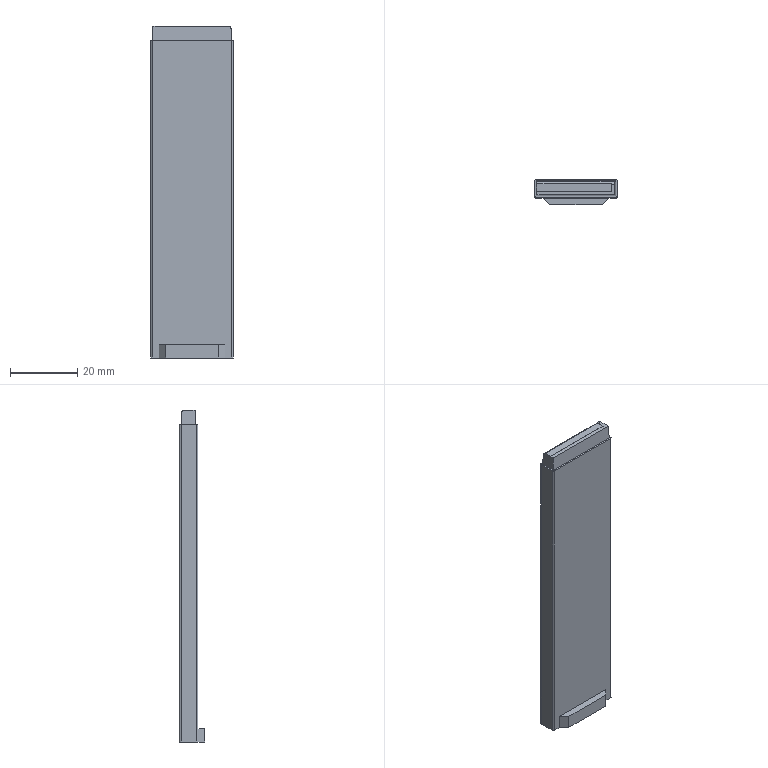Part | Creo | 1 solid | 23 faces | box 24.5 x 7.5 x 98.442 mm | volume 13224 mm3 | plane 18 | cylinder 5 | commonest cylinder face diameters 1 x4 2.01 x1
STEP:
#1=CARTESIAN_POINT('',(0.,0.,0.));
#2=DIRECTION('',(0.,0.,1.));
#3=DIRECTION('',(1.,0.,0.));
#4=AXIS2_PLACEMENT_3D('',#1,#2,#3);
#5=CARTESIAN_POINT('',(-20.598,-39.362,-54.09));
#6=VERTEX_POINT('',#5);
#7=CARTESIAN_POINT('',(-36.098,-39.362,-54.09));
#8=VERTEX_POINT('',#7);
#9=CARTESIAN_POINT('',(-20.598,-39.362,-54.09));
#10=DIRECTION('',(-1.,0.,0.));
#11=VECTOR('',#10,15.5);
#12=LINE('',#9,#11);
#13=EDGE_CURVE('',#6,#8,#12,.T.);
#14=ORIENTED_EDGE('',*,*,#13,.F.);
#15=CARTESIAN_POINT('',(-18.598,-37.362,-54.09));
#16=VERTEX_POINT('',#15);
#17=CARTESIAN_POINT('',(-18.598,-37.362,-54.09));
#18=DIRECTION('',(-0.7071,-0.7071,0.));
#19=VECTOR('',#18,2.828);
#20=LINE('',#17,#19);
#21=EDGE_CURVE('',#16,#6,#20,.T.);
#22=ORIENTED_EDGE('',*,*,#21,.F.);
#23=CARTESIAN_POINT('',(-16.598,-37.362,-54.09));
#24=VERTEX_POINT('',#23);
#25=CARTESIAN_POINT('',(-16.598,-37.362,-54.09));
#26=DIRECTION('',(-1.,0.,0.));
#27=VECTOR('',#26,2.);
#28=LINE('',#25,#27);
#29=EDGE_CURVE('',#24,#16,#28,.T.);
#30=ORIENTED_EDGE('',*,*,#29,.F.);
#31=CARTESIAN_POINT('',(-16.098,-36.862,-54.09));
#32=VERTEX_POINT('',#31);
#33=CARTESIAN_POINT('',(-16.598,-36.862,-54.09));
#34=DIRECTION('',(0.,0.,-1.));
#35=DIRECTION('',(1.,0.,0.));
#36=AXIS2_PLACEMENT_3D('',#33,#34,#35);
#37=CIRCLE('',#36,0.5);
#38=EDGE_CURVE('',#32,#24,#37,.T.);
#39=ORIENTED_EDGE('',*,*,#38,.F.);
#40=CARTESIAN_POINT('',(-16.098,-32.362,-54.09));
#41=VERTEX_POINT('',#40);
#42=CARTESIAN_POINT('',(-16.098,-32.362,-54.09));
#43=DIRECTION('',(0.,-1.,0.));
#44=VECTOR('',#43,4.5);
#45=LINE('',#42,#44);
#46=EDGE_CURVE('',#41,#32,#45,.T.);
#47=ORIENTED_EDGE('',*,*,#46,.F.);
#48=CARTESIAN_POINT('',(-16.598,-31.862,-54.09));
#49=VERTEX_POINT('',#48);
#50=CARTESIAN_POINT('',(-16.598,-32.362,-54.09));
#51=DIRECTION('',(0.,0.,-1.));
#52=DIRECTION('',(0.,1.,0.));
#53=AXIS2_PLACEMENT_3D('',#50,#51,#52);
#54=CIRCLE('',#53,0.5);
#55=EDGE_CURVE('',#49,#41,#54,.T.);
#56=ORIENTED_EDGE('',*,*,#55,.F.);
#57=CARTESIAN_POINT('',(-40.098,-31.862,-54.09));
#58=VERTEX_POINT('',#57);
#59=CARTESIAN_POINT('',(-40.098,-31.862,-54.09));
#60=DIRECTION('',(1.,0.,0.));
#61=VECTOR('',#60,23.5);
#62=LINE('',#59,#61);
#63=EDGE_CURVE('',#58,#49,#62,.T.);
#64=ORIENTED_EDGE('',*,*,#63,.F.);
#65=CARTESIAN_POINT('',(-40.598,-32.362,-54.09));
#66=VERTEX_POINT('',#65);
#67=CARTESIAN_POINT('',(-40.098,-32.362,-54.09));
#68=DIRECTION('',(0.,0.,-1.));
#69=DIRECTION('',(-1.,0.,0.));
#70=AXIS2_PLACEMENT_3D('',#67,#68,#69);
#71=CIRCLE('',#70,0.5);
#72=EDGE_CURVE('',#66,#58,#71,.T.);
#73=ORIENTED_EDGE('',*,*,#72,.F.);
#74=CARTESIAN_POINT('',(-40.598,-36.862,-54.09));
#75=VERTEX_POINT('',#74);
#76=CARTESIAN_POINT('',(-40.598,-36.862,-54.09));
#77=DIRECTION('',(0.,1.,0.));
#78=VECTOR('',#77,4.5);
#79=LINE('',#76,#78);
#80=EDGE_CURVE('',#75,#66,#79,.T.);
#81=ORIENTED_EDGE('',*,*,#80,.F.);
#82=CARTESIAN_POINT('',(-40.098,-37.362,-54.09));
#83=VERTEX_POINT('',#82);
#84=CARTESIAN_POINT('',(-40.098,-36.862,-54.09));
#85=DIRECTION('',(0.,0.,-1.));
#86=DIRECTION('',(0.,-1.,0.));
#87=AXIS2_PLACEMENT_3D('',#84,#85,#86);
#88=CIRCLE('',#87,0.5);
#89=EDGE_CURVE('',#83,#75,#88,.T.);
#90=ORIENTED_EDGE('',*,*,#89,.F.);
#91=CARTESIAN_POINT('',(-38.098,-37.362,-54.09));
#92=VERTEX_POINT('',#91);
#93=CARTESIAN_POINT('',(-38.098,-37.362,-54.09));
#94=DIRECTION('',(-1.,0.,0.));
#95=VECTOR('',#94,2.);
#96=LINE('',#93,#95);
#97=EDGE_CURVE('',#92,#83,#96,.T.);
#98=ORIENTED_EDGE('',*,*,#97,.F.);
#99=CARTESIAN_POINT('',(-36.098,-39.362,-54.09));
#100=DIRECTION('',(-0.7071,0.7071,0.));
#101=VECTOR('',#100,2.828);
#102=LINE('',#99,#101);
#103=EDGE_CURVE('',#8,#92,#102,.T.);
#104=ORIENTED_EDGE('',*,*,#103,.F.);
#105=EDGE_LOOP('',(#14,#22,#30,#39,#47,#56,#64,#73,#81,#90,#98,#104));
#106=FACE_OUTER_BOUND('',#105,.F.);
#107=CARTESIAN_POINT('',(0.,0.,-54.09));
#108=DIRECTION('',(0.,0.,-1.));
#109=DIRECTION('',(-1.,0.,0.));
#110=AXIS2_PLACEMENT_3D('',#107,#108,#109);
#111=PLANE('',#110);
#112=ADVANCED_FACE('',(#106),#111,.T.);
#113=CARTESIAN_POINT('',(-36.098,-39.362,-50.09));
#114=VERTEX_POINT('',#113);
#115=CARTESIAN_POINT('',(-20.598,-39.362,-50.09));
#116=VERTEX_POINT('',#115);
#117=CARTESIAN_POINT('',(-36.098,-39.362,-50.09));
#118=DIRECTION('',(1.,0.,0.));
#119=VECTOR('',#118,15.5);
#120=LINE('',#117,#119);
#121=EDGE_CURVE('',#114,#116,#120,.T.);
#122=ORIENTED_EDGE('',*,*,#121,.T.);
#123=CARTESIAN_POINT('',(-20.598,-39.362,-50.09));
#124=DIRECTION('',(0.,0.,-1.));
#125=VECTOR('',#124,4.);
#126=LINE('',#123,#125);
#127=EDGE_CURVE('',#116,#6,#126,.T.);
#128=ORIENTED_EDGE('',*,*,#127,.T.);
#129=ORIENTED_EDGE('',*,*,#13,.T.);
#130=CARTESIAN_POINT('',(-36.098,-39.362,-54.09));
#131=DIRECTION('',(0.,0.,1.));
#132=VECTOR('',#131,4.);
#133=LINE('',#130,#132);
#134=EDGE_CURVE('',#8,#114,#133,.T.);
#135=ORIENTED_EDGE('',*,*,#134,.T.);
#136=EDGE_LOOP('',(#122,#128,#129,#135));
#137=FACE_OUTER_BOUND('',#136,.F.);
#138=CARTESIAN_POINT('',(-28.348,-39.362,-54.09));
#139=DIRECTION('',(0.,-1.,0.));
#140=DIRECTION('',(0.,0.,-1.));
#141=AXIS2_PLACEMENT_3D('',#138,#139,#140);
#142=PLANE('',#141);
#143=ADVANCED_FACE('',(#137),#142,.T.);
#144=CARTESIAN_POINT('',(-18.598,-37.362,-50.09));
#145=VERTEX_POINT('',#144);
#146=CARTESIAN_POINT('',(-38.098,-37.362,-50.09));
#147=VERTEX_POINT('',#146);
#148=CARTESIAN_POINT('',(-18.598,-37.362,-50.09));
#149=DIRECTION('',(-1.,0.,0.));
#150=VECTOR('',#149,19.5);
#151=LINE('',#148,#150);
#152=EDGE_CURVE('',#145,#147,#151,.T.);
#153=ORIENTED_EDGE('',*,*,#152,.F.);
#154=CARTESIAN_POINT('',(-20.598,-39.362,-50.09));
#155=DIRECTION('',(0.7071,0.7071,0.));
#156=VECTOR('',#155,2.828);
#157=LINE('',#154,#156);
#158=EDGE_CURVE('',#116,#145,#157,.T.);
#159=ORIENTED_EDGE('',*,*,#158,.F.);
#160=ORIENTED_EDGE('',*,*,#121,.F.);
#161=CARTESIAN_POINT('',(-38.098,-37.362,-50.09));
#162=DIRECTION('',(0.7071,-0.7071,0.));
#163=VECTOR('',#162,2.828);
#164=LINE('',#161,#163);
#165=EDGE_CURVE('',#147,#114,#164,.T.);
#166=ORIENTED_EDGE('',*,*,#165,.F.);
#167=EDGE_LOOP('',(#153,#159,#160,#166));
#168=FACE_OUTER_BOUND('',#167,.F.);
#169=CARTESIAN_POINT('',(-28.348,-37.862,-50.09));
#170=DIRECTION('',(0.,0.,1.));
#171=DIRECTION('',(1.,0.,0.));
#172=AXIS2_PLACEMENT_3D('',#169,#170,#171);
#173=PLANE('',#172);
#174=ADVANCED_FACE('',(#168),#173,.T.);
#175=ORIENTED_EDGE('',*,*,#97,.T.);
#176=CARTESIAN_POINT('',(-40.098,-37.362,40.081));
#177=VERTEX_POINT('',#176);
#178=CARTESIAN_POINT('',(-40.098,-37.362,-54.09));
#179=DIRECTION('',(0.,0.,1.));
#180=VECTOR('',#179,94.171);
#181=LINE('',#178,#180);
#182=EDGE_CURVE('',#83,#177,#181,.T.);
#183=ORIENTED_EDGE('',*,*,#182,.T.);
#184=CARTESIAN_POINT('',(-16.598,-37.362,40.081));
#185=VERTEX_POINT('',#184);
#186=CARTESIAN_POINT('',(-40.098,-37.362,40.081));
#187=DIRECTION('',(1.,0.,0.));
#188=VECTOR('',#187,23.5);
#189=LINE('',#186,#188);
#190=EDGE_CURVE('',#177,#185,#189,.T.);
#191=ORIENTED_EDGE('',*,*,#190,.T.);
#192=CARTESIAN_POINT('',(-16.598,-37.362,40.081));
#193=DIRECTION('',(0.,0.,-1.));
#194=VECTOR('',#193,94.171);
#195=LINE('',#192,#194);
#196=EDGE_CURVE('',#185,#24,#195,.T.);
#197=ORIENTED_EDGE('',*,*,#196,.T.);
#198=ORIENTED_EDGE('',*,*,#29,.T.);
#199=CARTESIAN_POINT('',(-18.598,-37.362,-54.09));
#200=DIRECTION('',(0.,0.,1.));
#201=VECTOR('',#200,4.);
#202=LINE('',#199,#201);
#203=EDGE_CURVE('',#16,#145,#202,.T.);
#204=ORIENTED_EDGE('',*,*,#203,.T.);
#205=ORIENTED_EDGE('',*,*,#152,.T.);
#206=CARTESIAN_POINT('',(-38.098,-37.362,-50.09));
#207=DIRECTION('',(0.,0.,-1.));
#208=VECTOR('',#207,4.);
#209=LINE('',#206,#208);
#210=EDGE_CURVE('',#147,#92,#209,.T.);
#211=ORIENTED_EDGE('',*,*,#210,.T.);
#212=EDGE_LOOP('',(#175,#183,#191,#197,#198,#204,#205,#211));
#213=FACE_OUTER_BOUND('',#212,.F.);
#214=CARTESIAN_POINT('',(-40.598,-37.362,68.91));
#215=DIRECTION('',(0.,1.,0.));
#216=DIRECTION('',(0.,0.,1.));
#217=AXIS2_PLACEMENT_3D('',#214,#215,#216);
#218=PLANE('',#217);
#219=ADVANCED_FACE('',(#213),#218,.F.);
#220=CARTESIAN_POINT('',(-40.598,-36.862,40.081));
#221=VERTEX_POINT('',#220);
#222=CARTESIAN_POINT('',(-40.098,-36.862,40.081));
#223=DIRECTION('',(0.,0.,1.));
#224=DIRECTION('',(-1.,0.,0.));
#225=AXIS2_PLACEMENT_3D('',#222,#223,#224);
#226=CIRCLE('',#225,0.5);
#227=EDGE_CURVE('',#221,#177,#226,.T.);
#228=ORIENTED_EDGE('',*,*,#227,.T.);
#229=ORIENTED_EDGE('',*,*,#182,.F.);
#230=ORIENTED_EDGE('',*,*,#89,.T.);
#231=CARTESIAN_POINT('',(-40.598,-36.862,40.081));
#232=DIRECTION('',(0.,0.,-1.));
#233=VECTOR('',#232,94.171);
#234=LINE('',#231,#233);
#235=EDGE_CURVE('',#221,#75,#234,.T.);
#236=ORIENTED_EDGE('',*,*,#235,.F.);
#237=EDGE_LOOP('',(#228,#229,#230,#236));
#238=FACE_OUTER_BOUND('',#237,.F.);
#239=CARTESIAN_POINT('',(-40.098,-36.862,68.91));
#240=DIRECTION('',(0.,0.,-1.));
#241=DIRECTION('',(-1.,0.,0.));
#242=AXIS2_PLACEMENT_3D('',#239,#240,#241);
#243=CYLINDRICAL_SURFACE('',#242,0.5);
#244=ADVANCED_FACE('',(#238),#243,.T.);
#245=CARTESIAN_POINT('',(-16.598,-31.862,40.081));
#246=VERTEX_POINT('',#245);
#247=CARTESIAN_POINT('',(-40.098,-31.862,40.081));
#248=VERTEX_POINT('',#247);
#249=CARTESIAN_POINT('',(-16.598,-31.862,40.081));
#250=DIRECTION('',(-1.,0.,0.));
#251=VECTOR('',#250,23.5);
#252=LINE('',#249,#251);
#253=EDGE_CURVE('',#246,#248,#252,.T.);
#254=ORIENTED_EDGE('',*,*,#253,.F.);
#255=CARTESIAN_POINT('',(-16.098,-32.362,40.081));
#256=VERTEX_POINT('',#255);
#257=CARTESIAN_POINT('',(-16.598,-32.362,40.081));
#258=DIRECTION('',(0.,0.,1.));
#259=DIRECTION('',(1.,0.,0.));
#260=AXIS2_PLACEMENT_3D('',#257,#258,#259);
#261=CIRCLE('',#260,0.5);
#262=EDGE_CURVE('',#256,#246,#261,.T.);
#263=ORIENTED_EDGE('',*,*,#262,.F.);
#264=CARTESIAN_POINT('',(-16.098,-36.862,40.081));
#265=VERTEX_POINT('',#264);
#266=CARTESIAN_POINT('',(-16.098,-36.862,40.081));
#267=DIRECTION('',(0.,1.,0.));
#268=VECTOR('',#267,4.5);
#269=LINE('',#266,#268);
#270=EDGE_CURVE('',#265,#256,#269,.T.);
#271=ORIENTED_EDGE('',*,*,#270,.F.);
#272=CARTESIAN_POINT('',(-16.598,-36.862,40.081));
#273=DIRECTION('',(0.,0.,1.));
#274=DIRECTION('',(0.,-1.,0.));
#275=AXIS2_PLACEMENT_3D('',#272,#273,#274);
#276=CIRCLE('',#275,0.5);
#277=EDGE_CURVE('',#185,#265,#276,.T.);
#278=ORIENTED_EDGE('',*,*,#277,.F.);
#279=ORIENTED_EDGE('',*,*,#190,.F.);
#280=ORIENTED_EDGE('',*,*,#227,.F.);
#281=CARTESIAN_POINT('',(-40.598,-32.362,40.081));
#282=VERTEX_POINT('',#281);
#283=CARTESIAN_POINT('',(-40.598,-32.362,40.081));
#284=DIRECTION('',(0.,-1.,0.));
#285=VECTOR('',#284,4.5);
#286=LINE('',#283,#285);
#287=EDGE_CURVE('',#282,#221,#286,.T.);
#288=ORIENTED_EDGE('',*,*,#287,.F.);
#289=CARTESIAN_POINT('',(-40.098,-32.362,40.081));
#290=DIRECTION('',(0.,0.,1.));
#291=DIRECTION('',(0.,1.,0.));
#292=AXIS2_PLACEMENT_3D('',#289,#290,#291);
#293=CIRCLE('',#292,0.5);
#294=EDGE_CURVE('',#248,#282,#293,.T.);
#295=ORIENTED_EDGE('',*,*,#294,.F.);
#296=EDGE_LOOP('',(#254,#263,#271,#278,#279,#280,#288,#295));
#297=FACE_OUTER_BOUND('',#296,.F.);
#298=CARTESIAN_POINT('',(-16.598,-36.806,40.081));
#299=VERTEX_POINT('',#298);
#300=CARTESIAN_POINT('',(-40.14,-36.806,40.081));
#301=VERTEX_POINT('',#300);
#302=CARTESIAN_POINT('',(-16.598,-36.806,40.081));
#303=DIRECTION('',(-1.,0.,0.));
#304=VECTOR('',#303,23.542);
#305=LINE('',#302,#304);
#306=EDGE_CURVE('',#299,#301,#305,.T.);
#307=ORIENTED_EDGE('',*,*,#306,.F.);
#308=CARTESIAN_POINT('',(-16.598,-32.359,40.081));
#309=VERTEX_POINT('',#308);
#310=CARTESIAN_POINT('',(-16.598,-32.359,40.081));
#311=DIRECTION('',(0.,-1.,0.000000002));
#312=VECTOR('',#311,4.447);
#313=LINE('',#310,#312);
#314=EDGE_CURVE('',#309,#299,#313,.T.);
#315=ORIENTED_EDGE('',*,*,#314,.F.);
#316=CARTESIAN_POINT('',(-40.14,-32.359,40.081));
#317=VERTEX_POINT('',#316);
#318=CARTESIAN_POINT('',(-16.598,-32.359,40.081));
#319=DIRECTION('',(-1.,0.,0.));
#320=VECTOR('',#319,23.542);
#321=LINE('',#318,#320);
#322=EDGE_CURVE('',#309,#317,#321,.T.);
#323=ORIENTED_EDGE('',*,*,#322,.T.);
#324=CARTESIAN_POINT('',(-40.14,-32.359,40.081));
#325=DIRECTION('',(0.,-1.,0.000000002));
#326=VECTOR('',#325,4.447);
#327=LINE('',#324,#326);
#328=EDGE_CURVE('',#317,#301,#327,.T.);
#329=ORIENTED_EDGE('',*,*,#328,.T.);
#330=EDGE_LOOP('',(#307,#315,#323,#329));
#331=FACE_BOUND('',#330,.F.);
#332=CARTESIAN_POINT('',(-17.817,-88.35,40.081));
#333=DIRECTION('',(0.,0.,1.));
#334=DIRECTION('',(-1.,0.,0.));
#335=AXIS2_PLACEMENT_3D('',#332,#333,#334);
#336=PLANE('',#335);
#337=ADVANCED_FACE('',(#297,#331),#336,.T.);
#338=ORIENTED_EDGE('',*,*,#63,.T.);
#339=CARTESIAN_POINT('',(-16.598,-31.862,-54.09));
#340=DIRECTION('',(0.,0.,1.));
#341=VECTOR('',#340,94.171);
#342=LINE('',#339,#341);
#343=EDGE_CURVE('',#49,#246,#342,.T.);
#344=ORIENTED_EDGE('',*,*,#343,.T.);
#345=ORIENTED_EDGE('',*,*,#253,.T.);
#346=CARTESIAN_POINT('',(-40.098,-31.862,40.081));
#347=DIRECTION('',(0.,0.,-1.));
#348=VECTOR('',#347,94.171);
#349=LINE('',#346,#348);
#350=EDGE_CURVE('',#248,#58,#349,.T.);
#351=ORIENTED_EDGE('',*,*,#350,.T.);
#352=EDGE_LOOP('',(#338,#344,#345,#351));
#353=FACE_OUTER_BOUND('',#352,.F.);
#354=CARTESIAN_POINT('',(-16.098,-31.862,68.91));
#355=DIRECTION('',(0.,-1.,0.));
#356=DIRECTION('',(0.,0.,-1.));
#357=AXIS2_PLACEMENT_3D('',#354,#355,#356);
#358=PLANE('',#357);
#359=ADVANCED_FACE('',(#353),#358,.F.);
#360=ORIENTED_EDGE('',*,*,#262,.T.);
#361=ORIENTED_EDGE('',*,*,#343,.F.);
#362=ORIENTED_EDGE('',*,*,#55,.T.);
#363=CARTESIAN_POINT('',(-16.098,-32.362,40.081));
#364=DIRECTION('',(0.,0.,-1.));
#365=VECTOR('',#364,94.171);
#366=LINE('',#363,#365);
#367=EDGE_CURVE('',#256,#41,#366,.T.);
#368=ORIENTED_EDGE('',*,*,#367,.F.);
#369=EDGE_LOOP('',(#360,#361,#362,#368));
#370=FACE_OUTER_BOUND('',#369,.F.);
#371=CARTESIAN_POINT('',(-16.598,-32.362,68.91));
#372=DIRECTION('',(0.,0.,-1.));
#373=DIRECTION('',(-1.,0.,0.));
#374=AXIS2_PLACEMENT_3D('',#371,#372,#373);
#375=CYLINDRICAL_SURFACE('',#374,0.5);
#376=ADVANCED_FACE('',(#370),#375,.T.);
#377=ORIENTED_EDGE('',*,*,#367,.T.);
#378=ORIENTED_EDGE('',*,*,#46,.T.);
#379=CARTESIAN_POINT('',(-16.098,-36.862,-54.09));
#380=DIRECTION('',(0.,0.,1.));
#381=VECTOR('',#380,94.171);
#382=LINE('',#379,#381);
#383=EDGE_CURVE('',#32,#265,#382,.T.);
#384=ORIENTED_EDGE('',*,*,#383,.T.);
#385=ORIENTED_EDGE('',*,*,#270,.T.);
#386=EDGE_LOOP('',(#377,#378,#384,#385));
#387=FACE_OUTER_BOUND('',#386,.F.);
#388=CARTESIAN_POINT('',(-16.098,-37.362,68.91));
#389=DIRECTION('',(-1.,0.,0.));
#390=DIRECTION('',(0.,0.,1.));
#391=AXIS2_PLACEMENT_3D('',#388,#389,#390);
#392=PLANE('',#391);
#393=ADVANCED_FACE('',(#387),#392,.F.);
#394=ORIENTED_EDGE('',*,*,#277,.T.);
#395=ORIENTED_EDGE('',*,*,#383,.F.);
#396=ORIENTED_EDGE('',*,*,#38,.T.);
#397=ORIENTED_EDGE('',*,*,#196,.F.);
#398=EDGE_LOOP('',(#394,#395,#396,#397));
#399=FACE_OUTER_BOUND('',#398,.F.);
#400=CARTESIAN_POINT('',(-16.598,-36.862,68.91));
#401=DIRECTION('',(0.,0.,-1.));
#402=DIRECTION('',(-1.,0.,0.));
#403=AXIS2_PLACEMENT_3D('',#400,#401,#402);
#404=CYLINDRICAL_SURFACE('',#403,0.5);
#405=ADVANCED_FACE('',(#399),#404,.T.);
#406=ORIENTED_EDGE('',*,*,#294,.T.);
#407=CARTESIAN_POINT('',(-40.598,-32.362,-54.09));
#408=DIRECTION('',(0.,0.,1.));
#409=VECTOR('',#408,94.171);
#410=LINE('',#407,#409);
#411=EDGE_CURVE('',#66,#282,#410,.T.);
#412=ORIENTED_EDGE('',*,*,#411,.F.);
#413=ORIENTED_EDGE('',*,*,#72,.T.);
#414=ORIENTED_EDGE('',*,*,#350,.F.);
#415=EDGE_LOOP('',(#406,#412,#413,#414));
#416=FACE_OUTER_BOUND('',#415,.F.);
#417=CARTESIAN_POINT('',(-40.098,-32.362,68.91));
#418=DIRECTION('',(0.,0.,-1.));
#419=DIRECTION('',(-1.,0.,0.));
#420=AXIS2_PLACEMENT_3D('',#417,#418,#419);
#421=CYLINDRICAL_SURFACE('',#420,0.5);
#422=ADVANCED_FACE('',(#416),#421,.T.);
#423=ORIENTED_EDGE('',*,*,#235,.T.);
#424=ORIENTED_EDGE('',*,*,#80,.T.);
#425=ORIENTED_EDGE('',*,*,#411,.T.);
#426=ORIENTED_EDGE('',*,*,#287,.T.);
#427=EDGE_LOOP('',(#423,#424,#425,#426));
#428=FACE_OUTER_BOUND('',#427,.F.);
#429=CARTESIAN_POINT('',(-40.598,-31.862,68.91));
#430=DIRECTION('',(1.,0.,0.));
#431=DIRECTION('',(0.,0.,-1.));
#432=AXIS2_PLACEMENT_3D('',#429,#430,#431);
#433=PLANE('',#432);
#434=ADVANCED_FACE('',(#428),#433,.F.);
#435=CARTESIAN_POINT('',(-39.916,-36.582,44.352));
#436=VERTEX_POINT('',#435);
#437=CARTESIAN_POINT('',(-39.916,-36.582,44.352));
#438=DIRECTION('',(-0.05226,-0.05226,-0.9973));
#439=VECTOR('',#438,4.282);
#440=LINE('',#437,#439);
#441=EDGE_CURVE('',#436,#301,#440,.T.);
#442=ORIENTED_EDGE('',*,*,#441,.F.);
#443=CARTESIAN_POINT('',(-16.822,-36.582,44.352));
#444=VERTEX_POINT('',#443);
#445=CARTESIAN_POINT('',(-39.916,-36.582,44.352));
#446=DIRECTION('',(1.,0.,0.));
#447=VECTOR('',#446,23.094);
#448=LINE('',#445,#447);
#449=EDGE_CURVE('',#436,#444,#448,.T.);
#450=ORIENTED_EDGE('',*,*,#449,.T.);
#451=CARTESIAN_POINT('',(-16.822,-36.582,44.352));
#452=DIRECTION('',(0.05226,-0.05226,-0.9973));
#453=VECTOR('',#452,4.282);
#454=LINE('',#451,#453);
#455=EDGE_CURVE('',#444,#299,#454,.T.);
#456=ORIENTED_EDGE('',*,*,#455,.T.);
#457=ORIENTED_EDGE('',*,*,#306,.T.);
#458=EDGE_LOOP('',(#442,#450,#456,#457));
#459=FACE_OUTER_BOUND('',#458,.F.);
#460=CARTESIAN_POINT('',(-42.536,-36.593,44.151));
#461=DIRECTION('',(0.,-0.9986,0.05234));
#462=DIRECTION('',(1.,0.,0.));
#463=AXIS2_PLACEMENT_3D('',#460,#461,#462);
#464=PLANE('',#463);
#465=ADVANCED_FACE('',(#459),#464,.T.);
#466=CARTESIAN_POINT('',(-39.916,-35.502,44.352));
#467=VERTEX_POINT('',#466);
#468=CARTESIAN_POINT('',(-39.916,-35.502,44.352));
#469=DIRECTION('',(0.,-1.,0.));
#470=VECTOR('',#469,1.08);
#471=LINE('',#468,#470);
#472=EDGE_CURVE('',#467,#436,#471,.T.);
#473=ORIENTED_EDGE('',*,*,#472,.T.);
#474=ORIENTED_EDGE('',*,*,#441,.T.);
#475=ORIENTED_EDGE('',*,*,#328,.F.);
#476=CARTESIAN_POINT('',(-39.966,-32.525,43.397));
#477=VERTEX_POINT('',#476);
#478=CARTESIAN_POINT('',(-40.14,-32.359,40.081));
#479=DIRECTION('',(0.05227,-0.04991,0.9974));
#480=VECTOR('',#479,3.324);
#481=LINE('',#478,#480);
#482=EDGE_CURVE('',#317,#477,#481,.T.);
#483=ORIENTED_EDGE('',*,*,#482,.T.);
#484=CARTESIAN_POINT('',(-39.918,-33.248,44.312));
#485=VERTEX_POINT('',#484);
#486=CARTESIAN_POINT('',(-39.922,-33.019,44.245));
#487=CARTESIAN_POINT('',(-39.934,-32.703,43.999));
#488=CARTESIAN_POINT('',(-39.954,-32.537,43.635));
#489=CARTESIAN_POINT('',(-39.966,-32.525,43.397));
#490=B_SPLINE_CURVE_WITH_KNOTS('',3,(#484,#486,#487,#488,#489),.UNSPECIFIED.,.F.,.F.,(4,1,4),(0.,0.5,1.),.UNSPECIFIED.);
#491=EDGE_CURVE('',#485,#477,#490,.T.);
#492=ORIENTED_EDGE('',*,*,#491,.F.);
#493=CARTESIAN_POINT('',(-39.918,-35.502,44.312));
#494=VERTEX_POINT('',#493);
#495=CARTESIAN_POINT('',(-39.918,-35.502,44.312));
#496=DIRECTION('',(0.,1.,0.));
#497=VECTOR('',#496,2.253);
#498=LINE('',#495,#497);
#499=EDGE_CURVE('',#494,#485,#498,.T.);
#500=ORIENTED_EDGE('',*,*,#499,.F.);
#501=CARTESIAN_POINT('',(-39.918,-35.502,44.312));
#502=DIRECTION('',(0.05234,0.,0.9986));
#503=VECTOR('',#502,0.04005);
#504=LINE('',#501,#503);
#505=EDGE_CURVE('',#494,#467,#504,.T.);
#506=ORIENTED_EDGE('',*,*,#505,.T.);
#507=EDGE_LOOP('',(#473,#474,#475,#483,#492,#500,#506));
#508=FACE_OUTER_BOUND('',#507,.F.);
#509=CARTESIAN_POINT('',(-39.926,-91.965,44.151));
#510=DIRECTION('',(0.9986,0.,-0.05234));
#511=DIRECTION('',(0.,1.,0.));
#512=AXIS2_PLACEMENT_3D('',#509,#510,#511);
#513=PLANE('',#512);
#514=ADVANCED_FACE('',(#508),#513,.F.);
#515=CARTESIAN_POINT('',(-17.902,-33.529,44.352));
#516=VERTEX_POINT('',#515);
#517=CARTESIAN_POINT('',(-17.902,-35.502,44.352));
#518=VERTEX_POINT('',#517);
#519=CARTESIAN_POINT('',(-17.902,-33.529,44.352));
#520=DIRECTION('',(0.,-1.,0.));
#521=VECTOR('',#520,1.973);
#522=LINE('',#519,#521);
#523=EDGE_CURVE('',#516,#518,#522,.T.);
#524=ORIENTED_EDGE('',*,*,#523,.F.);
#525=CARTESIAN_POINT('',(-16.822,-33.529,44.352));
#526=VERTEX_POINT('',#525);
#527=CARTESIAN_POINT('',(-17.902,-33.529,44.352));
#528=DIRECTION('',(1.,0.,0.));
#529=VECTOR('',#528,1.08);
#530=LINE('',#527,#529);
#531=EDGE_CURVE('',#516,#526,#530,.T.);
#532=ORIENTED_EDGE('',*,*,#531,.T.);
#533=CARTESIAN_POINT('',(-16.822,-36.582,44.352));
#534=DIRECTION('',(0.,1.,0.));
#535=VECTOR('',#534,3.053);
#536=LINE('',#533,#535);
#537=EDGE_CURVE('',#444,#526,#536,.T.);
#538=ORIENTED_EDGE('',*,*,#537,.F.);
#539=ORIENTED_EDGE('',*,*,#449,.F.);
#540=ORIENTED_EDGE('',*,*,#472,.F.);
#541=CARTESIAN_POINT('',(-17.902,-35.502,44.352));
#542=DIRECTION('',(-1.,0.,0.));
#543=VECTOR('',#542,22.014);
#544=LINE('',#541,#543);
#545=EDGE_CURVE('',#518,#467,#544,.T.);
#546=ORIENTED_EDGE('',*,*,#545,.F.);
#547=EDGE_LOOP('',(#524,#532,#538,#539,#540,#546));
#548=FACE_OUTER_BOUND('',#547,.F.);
#549=CARTESIAN_POINT('',(-16.811,-32.572,44.352));
#550=DIRECTION('',(0.,0.,1.));
#551=DIRECTION('',(0.,1.,0.));
#552=AXIS2_PLACEMENT_3D('',#549,#550,#551);
#553=PLANE('',#552);
#554=ADVANCED_FACE('',(#548),#553,.T.);
#555=CARTESIAN_POINT('',(-17.902,-33.248,44.312));
#556=VERTEX_POINT('',#555);
#557=CARTESIAN_POINT('',(-17.902,-33.529,43.346));
#558=DIRECTION('',(-1.,0.,0.));
#559=DIRECTION('',(0.,0.,1.));
#560=AXIS2_PLACEMENT_3D('',#557,#558,#559);
#561=CIRCLE('',#560,1.005);
#562=EDGE_CURVE('',#516,#556,#561,.T.);
#563=ORIENTED_EDGE('',*,*,#562,.F.);
#564=ORIENTED_EDGE('',*,*,#523,.T.);
#565=CARTESIAN_POINT('',(-17.902,-35.502,44.312));
#566=VERTEX_POINT('',#565);
#567=CARTESIAN_POINT('',(-17.902,-35.502,44.352));
#568=DIRECTION('',(0.,0.,-1.));
#569=VECTOR('',#568,0.04);
#570=LINE('',#567,#569);
#571=EDGE_CURVE('',#518,#566,#570,.T.);
#572=ORIENTED_EDGE('',*,*,#571,.T.);
#573=CARTESIAN_POINT('',(-17.902,-33.248,44.312));
#574=DIRECTION('',(0.,-1.,0.));
#575=VECTOR('',#574,2.253);
#576=LINE('',#573,#575);
#577=EDGE_CURVE('',#556,#566,#576,.T.);
#578=ORIENTED_EDGE('',*,*,#577,.F.);
#579=EDGE_LOOP('',(#563,#564,#572,#578));
#580=FACE_OUTER_BOUND('',#579,.F.);
#581=CARTESIAN_POINT('',(-17.902,-33.526,45.151));
#582=DIRECTION('',(1.,0.,0.));
#583=DIRECTION('',(0.,0.,-1.));
#584=AXIS2_PLACEMENT_3D('',#581,#582,#583);
#585=PLANE('',#584);
#586=ADVANCED_FACE('',(#580),#585,.F.);
#587=ORIENTED_EDGE('',*,*,#562,.T.);
#588=CARTESIAN_POINT('',(-39.918,-33.248,44.312));
#589=DIRECTION('',(1.,0.,0.));
#590=VECTOR('',#589,22.016);
#591=LINE('',#588,#590);
#592=EDGE_CURVE('',#485,#556,#591,.T.);
#593=ORIENTED_EDGE('',*,*,#592,.F.);
#594=ORIENTED_EDGE('',*,*,#491,.T.);
#595=CARTESIAN_POINT('',(-16.772,-32.525,43.397));
#596=VERTEX_POINT('',#595);
#597=CARTESIAN_POINT('',(-16.772,-32.525,43.397));
#598=DIRECTION('',(-1.,0.,0.));
#599=VECTOR('',#598,23.194);
#600=LINE('',#597,#599);
#601=EDGE_CURVE('',#596,#477,#600,.T.);
#602=ORIENTED_EDGE('',*,*,#601,.F.);
#603=CARTESIAN_POINT('',(-16.822,-33.529,44.352));
#604=CARTESIAN_POINT('',(-16.822,-33.369,44.352));
#605=CARTESIAN_POINT('',(-16.818,-33.114,44.285));
#606=CARTESIAN_POINT('',(-16.808,-32.822,44.089));
#607=CARTESIAN_POINT('',(-16.793,-32.612,43.807));
#608=CARTESIAN_POINT('',(-16.78,-32.533,43.556));
#609=B_SPLINE_CURVE_WITH_KNOTS('',3,(#603,#604,#605,#606,#607,#608,#595),.UNSPECIFIED.,.F.,.F.,(4,1,1,1,4),(0.,0.25,0.5,0.75,1.),.UNSPECIFIED.);
#610=EDGE_CURVE('',#526,#596,#609,.T.);
#611=ORIENTED_EDGE('',*,*,#610,.F.);
#612=ORIENTED_EDGE('',*,*,#531,.F.);
#613=EDGE_LOOP('',(#587,#593,#594,#602,#611,#612));
#614=FACE_OUTER_BOUND('',#613,.F.);
#615=CARTESIAN_POINT('',(-16.811,-33.529,43.346));
#616=DIRECTION('',(-1.,0.,0.));
#617=DIRECTION('',(0.,0.,1.));
#618=AXIS2_PLACEMENT_3D('',#615,#616,#617);
#619=CYLINDRICAL_SURFACE('',#618,1.005);
#620=ADVANCED_FACE('',(#614),#619,.T.);
#621=ORIENTED_EDGE('',*,*,#499,.T.);
#622=ORIENTED_EDGE('',*,*,#592,.T.);
#623=ORIENTED_EDGE('',*,*,#577,.T.);
#624=CARTESIAN_POINT('',(-17.902,-35.502,44.312));
#625=DIRECTION('',(-1.,0.,0.));
#626=VECTOR('',#625,22.016);
#627=LINE('',#624,#626);
#628=EDGE_CURVE('',#566,#494,#627,.T.);
#629=ORIENTED_EDGE('',*,*,#628,.T.);
#630=EDGE_LOOP('',(#621,#622,#623,#629));
#631=FACE_OUTER_BOUND('',#630,.F.);
#632=CARTESIAN_POINT('',(-16.811,-32.572,44.312));
#633=DIRECTION('',(0.,0.,1.));
#634=DIRECTION('',(0.,1.,0.));
#635=AXIS2_PLACEMENT_3D('',#632,#633,#634);
#636=PLANE('',#635);
#637=ADVANCED_FACE('',(#631),#636,.T.);
#638=ORIENTED_EDGE('',*,*,#545,.T.);
#639=ORIENTED_EDGE('',*,*,#505,.F.);
#640=ORIENTED_EDGE('',*,*,#628,.F.);
#641=ORIENTED_EDGE('',*,*,#571,.F.);
#642=EDGE_LOOP('',(#638,#639,#640,#641));
#643=FACE_OUTER_BOUND('',#642,.F.);
#644=CARTESIAN_POINT('',(-17.852,-35.502,45.151));
#645=DIRECTION('',(0.,-1.,0.));
#646=DIRECTION('',(0.,0.,-1.));
#647=AXIS2_PLACEMENT_3D('',#644,#645,#646);
#648=PLANE('',#647);
#649=ADVANCED_FACE('',(#643),#648,.F.);
#650=ORIENTED_EDGE('',*,*,#601,.T.);
#651=ORIENTED_EDGE('',*,*,#482,.F.);
#652=ORIENTED_EDGE('',*,*,#322,.F.);
#653=CARTESIAN_POINT('',(-16.772,-32.525,43.397));
#654=DIRECTION('',(0.05227,0.04991,-0.9974));
#655=VECTOR('',#654,3.324);
#656=LINE('',#653,#655);
#657=EDGE_CURVE('',#596,#309,#656,.T.);
#658=ORIENTED_EDGE('',*,*,#657,.F.);
#659=EDGE_LOOP('',(#650,#651,#652,#658));
#660=FACE_OUTER_BOUND('',#659,.F.);
#661=CARTESIAN_POINT('',(-42.536,-32.563,44.152));
#662=DIRECTION('',(0.,0.9988,0.04998));
#663=DIRECTION('',(-1.,0.,0.));
#664=AXIS2_PLACEMENT_3D('',#661,#662,#663);
#665=PLANE('',#664);
#666=ADVANCED_FACE('',(#660),#665,.T.);
#667=ORIENTED_EDGE('',*,*,#657,.T.);
#668=ORIENTED_EDGE('',*,*,#314,.T.);
#669=ORIENTED_EDGE('',*,*,#455,.F.);
#670=ORIENTED_EDGE('',*,*,#537,.T.);
#671=ORIENTED_EDGE('',*,*,#610,.T.);
#672=EDGE_LOOP('',(#667,#668,#669,#670,#671));
#673=FACE_OUTER_BOUND('',#672,.F.);
#674=CARTESIAN_POINT('',(-16.811,-91.965,44.151));
#675=DIRECTION('',(0.9986,0.,0.05234));
#676=DIRECTION('',(0.,1.,0.));
#677=AXIS2_PLACEMENT_3D('',#674,#675,#676);
#678=PLANE('',#677);
#679=ADVANCED_FACE('',(#673),#678,.T.);
#680=ORIENTED_EDGE('',*,*,#21,.T.);
#681=ORIENTED_EDGE('',*,*,#127,.F.);
#682=ORIENTED_EDGE('',*,*,#158,.T.);
#683=ORIENTED_EDGE('',*,*,#203,.F.);
#684=EDGE_LOOP('',(#680,#681,#682,#683));
#685=FACE_OUTER_BOUND('',#684,.F.);
#686=CARTESIAN_POINT('',(-20.598,-39.362,-54.09));
#687=DIRECTION('',(-0.7071,0.7071,0.));
#688=DIRECTION('',(0.,0.,1.));
#689=AXIS2_PLACEMENT_3D('',#686,#687,#688);
#690=PLANE('',#689);
#691=ADVANCED_FACE('',(#685),#690,.F.);
#692=ORIENTED_EDGE('',*,*,#103,.T.);
#693=ORIENTED_EDGE('',*,*,#210,.F.);
#694=ORIENTED_EDGE('',*,*,#165,.T.);
#695=ORIENTED_EDGE('',*,*,#134,.F.);
#696=EDGE_LOOP('',(#692,#693,#694,#695));
#697=FACE_OUTER_BOUND('',#696,.F.);
#698=CARTESIAN_POINT('',(-38.098,-37.362,-54.09));
#699=DIRECTION('',(0.7071,0.7071,0.));
#700=DIRECTION('',(0.,0.,1.));
#701=AXIS2_PLACEMENT_3D('',#698,#699,#700);
#702=PLANE('',#701);
#703=ADVANCED_FACE('',(#697),#702,.F.);
#704=CLOSED_SHELL('',(#112,#143,#174,#219,#244,#337,#359,#376,#393,#405,#422,#434,#465,#514,#554,#586,#620,#637,#649,#666,#679,#691,#703));
#705=MANIFOLD_SOLID_BREP('',#704);
#706=(LENGTH_UNIT()NAMED_UNIT(*)SI_UNIT(.MILLI.,.METRE.));
#707=UNCERTAINTY_MEASURE_WITH_UNIT(LENGTH_MEASURE(0.01017),#706,'','');
#708=(NAMED_UNIT(*)PLANE_ANGLE_UNIT()SI_UNIT($,.RADIAN.));
#709=PLANE_ANGLE_MEASURE_WITH_UNIT(PLANE_ANGLE_MEASURE(0.01745),#708);
#710=(CONVERSION_BASED_UNIT('DEGREE',#709)NAMED_UNIT(*)PLANE_ANGLE_UNIT());
#711=(NAMED_UNIT(*)SI_UNIT($,.STERADIAN.)SOLID_ANGLE_UNIT());
#712=(GEOMETRIC_REPRESENTATION_CONTEXT(3)GLOBAL_UNCERTAINTY_ASSIGNED_CONTEXT((#707))GLOBAL_UNIT_ASSIGNED_CONTEXT((#706,#710,#711))REPRESENTATION_CONTEXT('',''));
#713=ADVANCED_BREP_SHAPE_REPRESENTATION('',(#4,#705),#712);